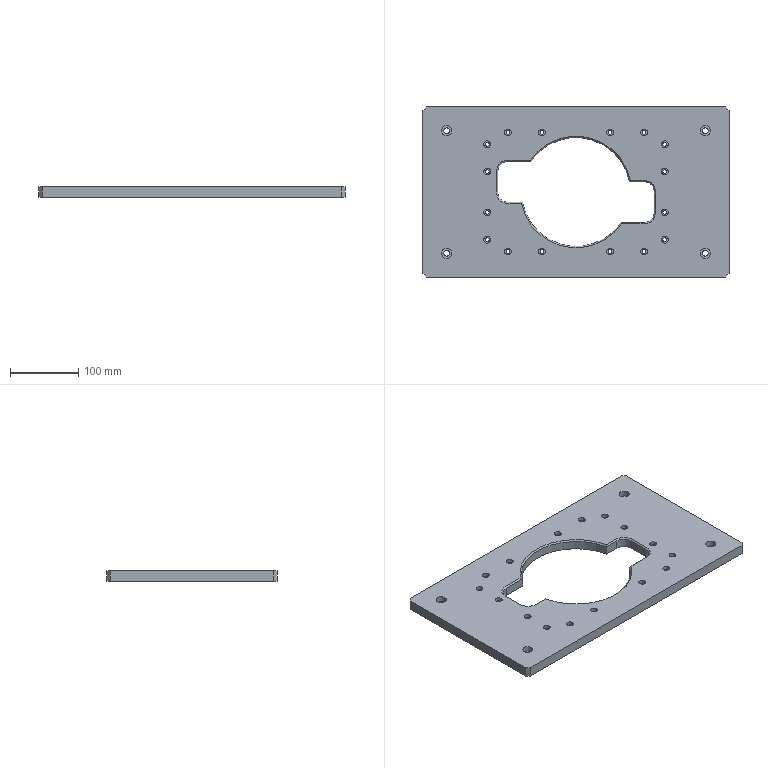Part | STEP file | 10-14 lift fixed platform | 1 solid | 146 faces | box 450 x 250 x 15 mm | volume 1290007 mm3 | cylinder 94 | plane 46 | cone 6 | commonest cylinder face diameters 5.5 x32 10 x32 8.4 x8 15 x8 40 x8 30 x4